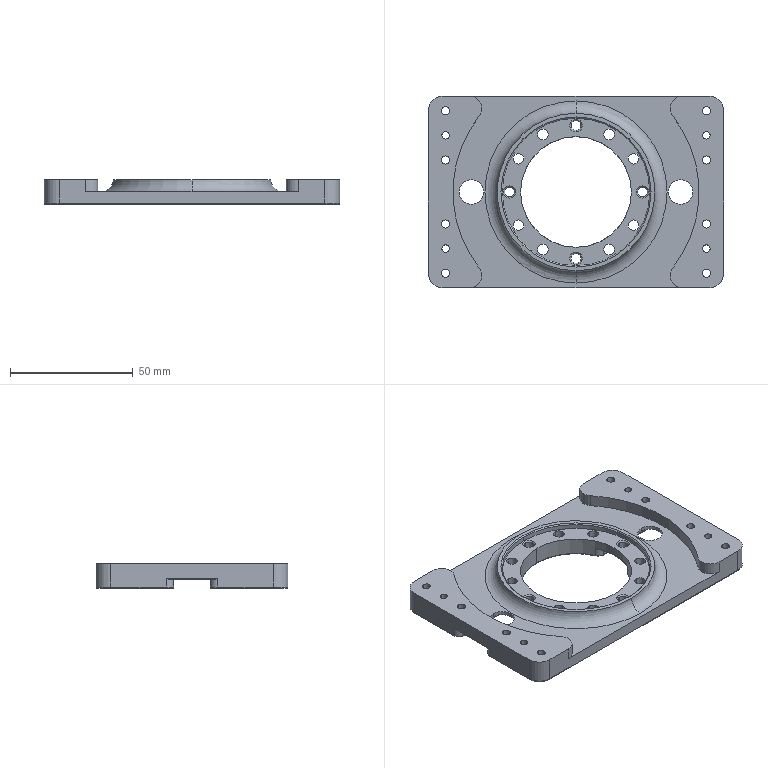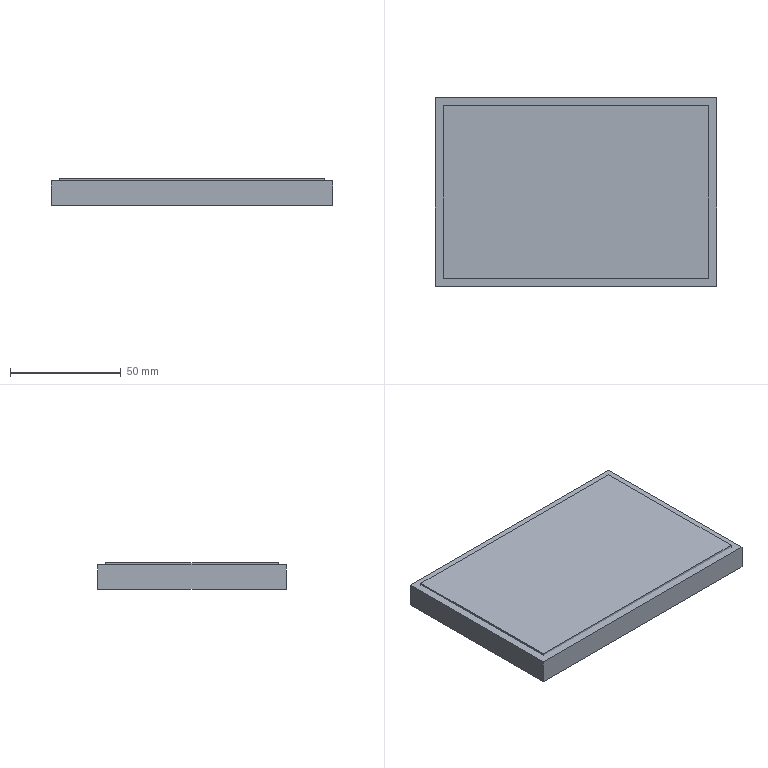CAM job | NX | 3+2 milling, drilling | part box 120 x 78 x 10 mm | stock box 127 x 85 x 12 mm
Tools:
number,name,description,diameter,corner_radius,flute_length,length,flutes
19,D80,Milling Tool-5 Parameters,80.0,0.0,50.0,75.0,2
1,D6A45,Milling Tool-5 Parameters,6.0,0.0,50.0,75.0,2
3,3.3ZT,Drilling Tool,3.3,0.0,35.0,50.0,2
16,4.3ZT,Drilling Tool,4.3,0.0,35.0,50.0,2
2,2.5ZT,Drilling Tool,2.5,0.0,35.0,50.0,2
15,D10,Milling Tool-5 Parameters,10.0,0.0,50.0,75.0,2
14,D10JING,Milling Tool-5 Parameters,10.0,0.0,50.0,75.0,2
12,D6,Milling Tool-5 Parameters,6.0,0.0,50.0,75.0,2
17,D3,Milling Tool-5 Parameters,3.0,0.0,50.0,75.0,2
18,D2,Milling Tool-5 Parameters,2.0,0.0,50.0,75.0,2
24,D2R0.5,Milling Tool-5 Parameters,2.0,0.5,50.0,75.0,2
5,D4R0.5,Milling Tool-5 Parameters,4.0,0.5,50.0,75.0,2
Operations:
program,operation,operation_type,tool,method,geometry_group,spindle_rpm,surface_speed,feed_per_tooth,feed_cut,feed_plunge,cut_length_mm,path_length_mm,cut_time_min,machine_time_min
1,FLOOR_WALL,VolumeBased25DMillingOperation,D80,METHOD,A,6500.0,1633.0,0.1154,1500.0,100.0,685.997,739.997,0.4573,0.4627
1,DRILLING,Operation,D6A45,METHOD,A,5000.0,94.0,0.035,350.0,0.0,80.0,648.858,0.2286,0.2855
1,DRILLING_COPY_1,Operation,D6A45,METHOD,A,5000.0,94.0,0.035,350.0,0.0,33.0,392.901,0.0943,0.1303
1,DRILLING_COPY,Operation,3.3ZT,METHOD,A,2000.0,20.0,0.045,180.0,0.0,119.931,560.145,0.6663,0.7103
1,DRILLING_COPY_COPY_1,Operation,3.3ZT,METHOD,A,2000.0,20.0,0.045,180.0,0.0,59.966,303.836,0.3331,0.3575
1,DRILLING_COPY_COPY_1_COPY,Operation,2.5ZT,METHOD,A,2000.0,15.0,0.03,120.0,0.0,59.004,385.247,0.4917,0.5243
1,DRILLING_COPY_COPY,Operation,4.3ZT,METHOD,A,2000.0,20.0,0.045,180.0,0.0,122.335,464.346,0.6796,0.7138
1,ADAPTIVE_MILLING,CavityMilling,D10,METHOD,A,9500.0,298.0,0.1579,3000.0,1000.0,3935.022,4138.246,1.81,1.831
1,ADAPTIVE_MILLING_COPY,CavityMilling,D10,METHOD,A,9500.0,298.0,0.1579,3000.0,1000.0,2697.457,3093.517,1.579,1.619
1,ADAPTIVE_MILLING_COPY_COPY,CavityMilling,D10,METHOD,A,9500.0,298.0,0.1579,3000.0,1000.0,4566.718,4859.221,2.017,2.046
1,ZLEVEL_PROFILE_COPY_1_COPY_COPY_1,ZLevelMilling,D10JING,METHOD,A,9500.0,298.0,0.0632,1200.0,1000.0,542.303,806.213,0.4532,0.4796
1,FLOOR_WALL_COPY,VolumeBased25DMillingOperation,D10JING,METHOD,A,9500.0,298.0,0.0789,1500.0,1000.0,445.479,1013.823,0.329,0.3858
1,HOLE_MILLING,CylinderMilling,D6,METHOD,A,9500.0,179.0,0.0737,1400.0,100.0,759.957,1584.473,0.5428,0.6253
1,ZLEVEL_PROFILE,ZLevelMilling,D6,METHOD,A,9500.0,179.0,0.1053,2000.0,100.0,594.319,2022.32,0.2972,0.44
1,FLOOR_WALL_COPY_COPY,VolumeBased25DMillingOperation,D6,METHOD,A,9500.0,298.0,0.0789,1500.0,1000.0,777.059,1193.896,0.521,0.5627
1,HOLE_MILLING_1,CylinderMilling,D3,METHOD,A,9500.0,89.0,0.0658,1250.0,100.0,466.596,1287.141,0.3733,0.4553
1,HOLE_MILLING_1_COPY,CylinderMilling,D2,METHOD,A,9500.0,89.0,0.0658,1250.0,100.0,451.489,943.489,0.3612,0.4104
1,PLANAR_MILL_COPY_COPY_COPY_COPY_COPY_COPY_1,PlanarMilling,D6A45,METHOD,A,9500.0,179.0,0.0658,1250.0,100.0,619.611,2156.337,0.4957,0.6494
1,PLANAR_MILL_COPY_COPY_COPY_COPY_COPY_COPY_1_COPY,PlanarMilling,D6A45,METHOD,A,9500.0,179.0,0.0658,1250.0,100.0,85.723,438.373,0.0686,0.1038
1,ZLEVEL_PROFILE_1,ZLevelMilling,D2R0.5,METHOD,A,9500.0,59.0,0.1316,2500.0,100.0,9360.243,9612.652,3.744,3.769
1,ZLEVEL_PROFILE_1_COPY,ZLevelMilling,D2R0.5,METHOD,A,9500.0,59.0,0.1316,2500.0,100.0,1089.718,1477.213,0.4359,0.4746
1,刀补17,CylinderMilling,D3,METHOD,A,9500.0,89.0,0.0658,1250.0,100.0,99.026,919.571,0.0792,0.1613
1,刀补18,CylinderMilling,D2,METHOD,A,9500.0,89.0,0.0658,1250.0,100.0,56.156,548.156,0.0449,0.0941
2,FLOOR_WALL_COPY_1,VolumeBased25DMillingOperation,D80,METHOD,B,6500.0,1633.0,0.1154,1500.0,100.0,1323.994,1644.973,0.8827,0.9148
2,ADAPTIVE_MILLING_COPY_1,CavityMilling,D10,METHOD,B,9500.0,298.0,0.1579,3000.0,1000.0,10700.24,10909.022,3.867,3.888
2,HOLE_MILLING_2,CylinderMilling,D10,METHOD,B,9500.0,298.0,0.1316,2500.0,100.0,1183.836,1250.439,0.4735,0.4802
2,FLOOR_WALL_COPY_COPY_COPY,VolumeBased25DMillingOperation,D6,METHOD,B,9500.0,298.0,0.0789,1500.0,1000.0,1386.903,2110.573,0.937,1.009
2,ZLEVEL_PROFILE_1_COPY_1,ZLevelMilling,D4R0.5,METHOD,B,9500.0,59.0,0.1316,2500.0,100.0,16289.637,16352.637,6.516,6.522
2,PLANAR_MILL_COPY_COPY_COPY_COPY_COPY_COPY_1_COPY_1,PlanarMilling,D6A45,METHOD,B,9500.0,179.0,0.0658,1250.0,100.0,725.456,1906.99,0.5804,0.6985
2,PLANAR_MILL_COPY_COPY_COPY_COPY_COPY_COPY_1_COPY_1_COPY,PlanarMilling,D6A45,METHOD,B,9500.0,179.0,0.0658,1250.0,100.0,190.448,249.448,0.1524,0.1583
2,PLANAR_MILL_COPY_COPY_COPY_COPY_COPY_COPY_1_COPY_1_COPY_COPY,PlanarMilling,D6A45,METHOD,B,9500.0,179.0,0.0658,1250.0,100.0,140.183,203.983,0.1121,0.1185
2,PLANAR_MILL_COPY_COPY_COPY_COPY_COPY_COPY_1_COPY_1_COPY_COPY_COPY,PlanarMilling,D6A45,METHOD,B,9500.0,179.0,0.0658,1250.0,100.0,227.71,721.484,0.1822,0.2315
2,刀补12,CylinderMilling,D6,METHOD,B,9500.0,179.0,0.0632,1200.0,100.0,230.588,292.488,0.1922,0.1983
3,HOLE_MILLING_1_COPY_1,CylinderMilling,D3,METHOD,C,9500.0,89.0,0.0658,1250.0,100.0,492.437,726.437,0.3939,0.4173
3,ZLEVEL_PROFILE_COPY_1_COPY_COPY_1_COPY,ZLevelMilling,D6A45,METHOD,C,9500.0,179.0,0.0632,1200.0,1000.0,213.126,418.729,0.1794,0.1999
3,刀补17_COPY,CylinderMilling,D3,METHOD,C,9500.0,89.0,0.0658,1250.0,100.0,72.308,306.308,0.0578,0.0812